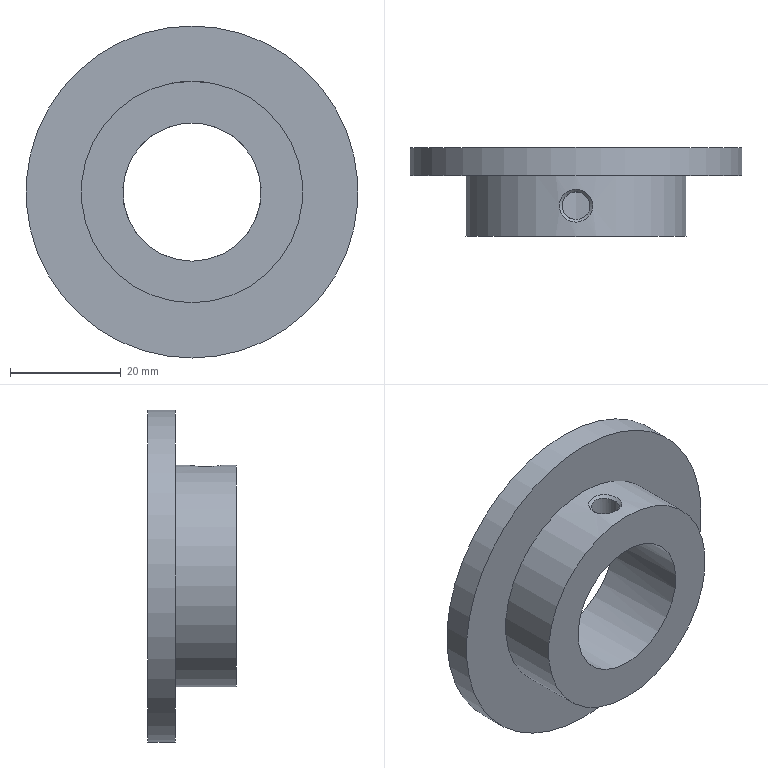Part | STEP file | 冲床-300配套压波_id586_x_t | 1 solid | 9 faces | box 60 x 16 x 60 mm | volume 19955 mm3 | cylinder 4 | plane 3 | spline 2 | commonest cylinder face diameters 5 x1 25 x1 40 x1 60 x1